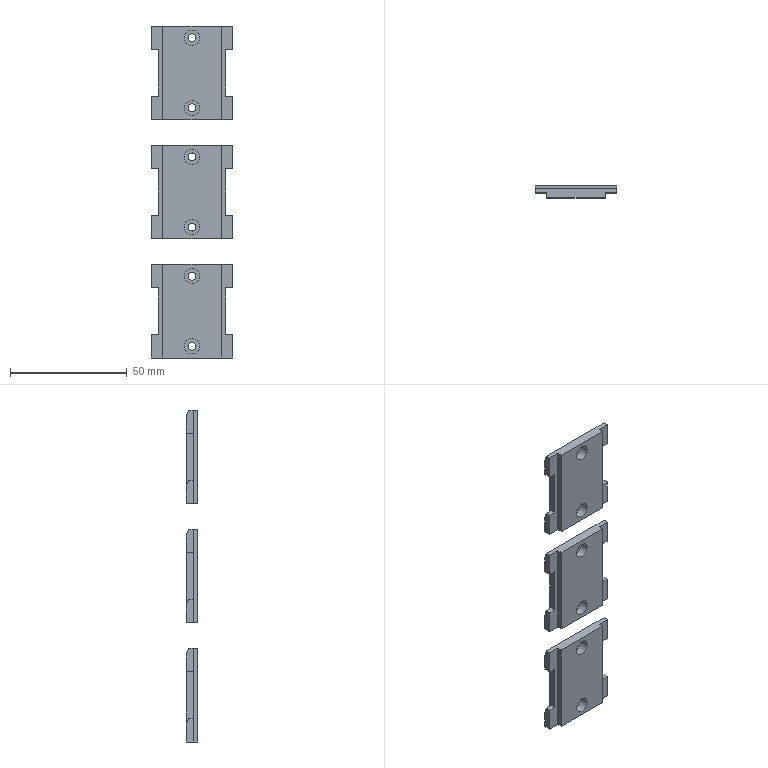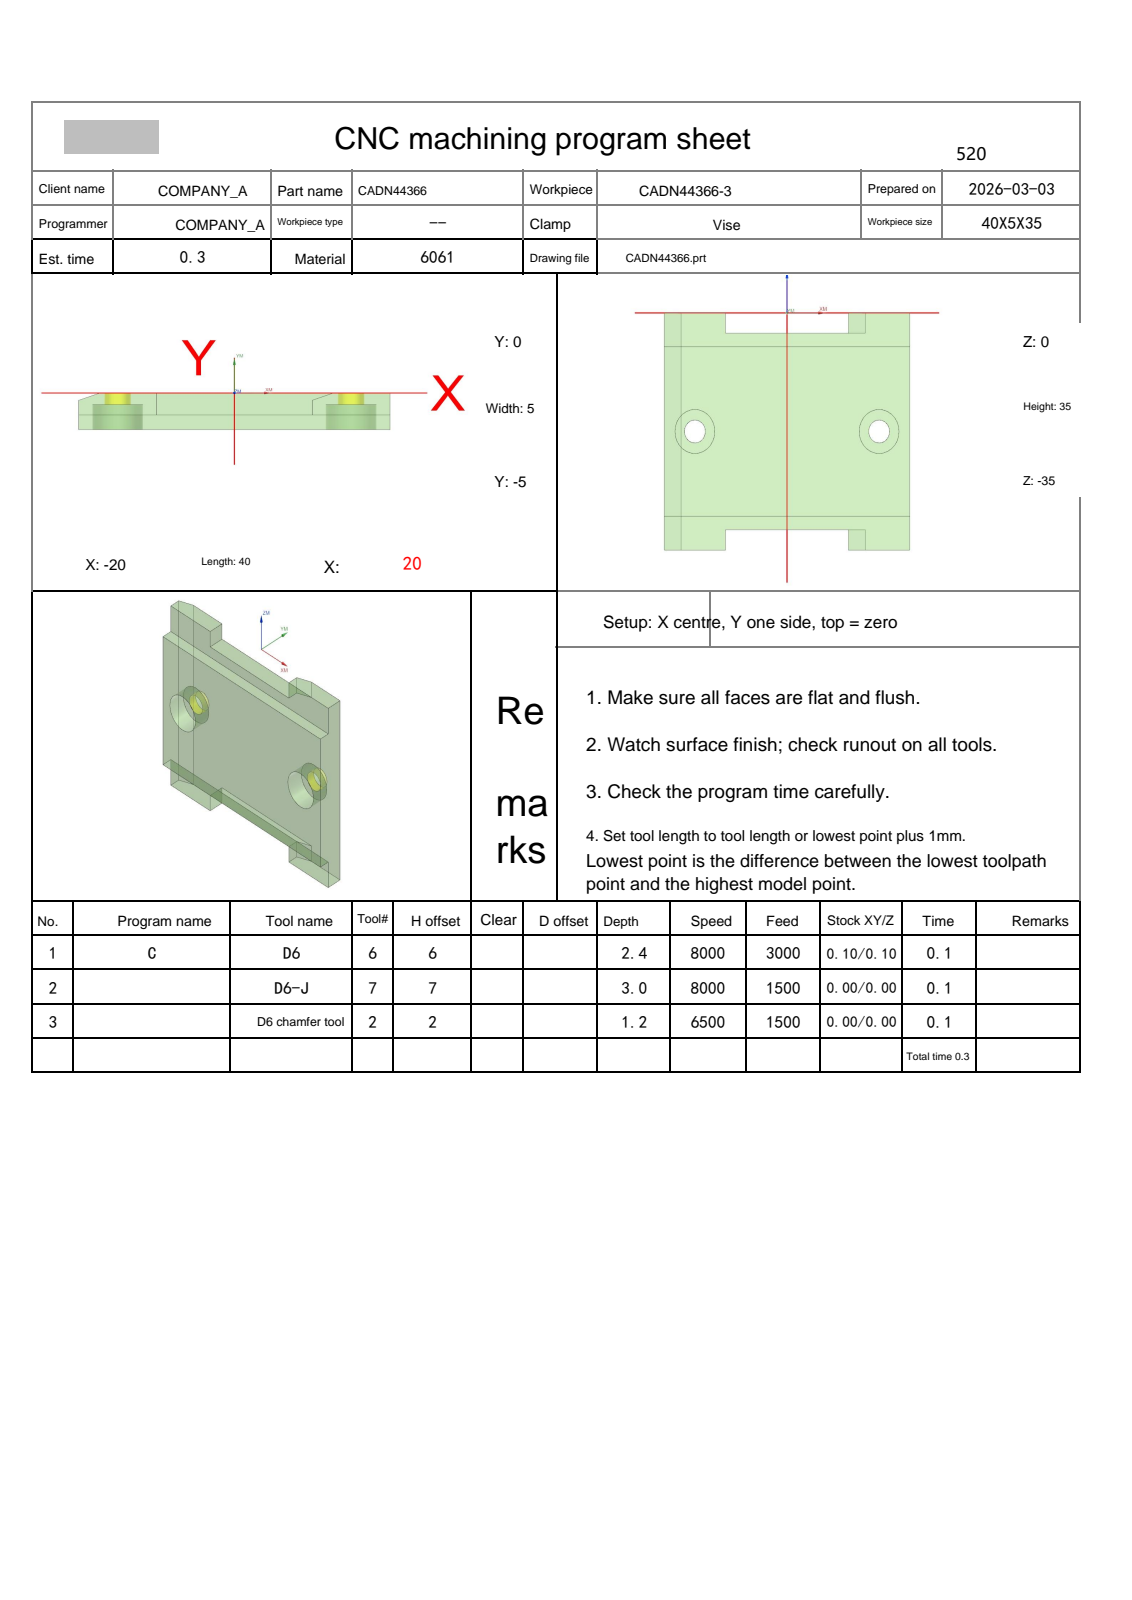NC program | NX | posted by the shop | part box 35 x 5 x 142 mm
Whole program:
%
O0001
(Machine time: 0.80 MIN)
(===Total Tool:3===)
(T6=D6      D=6.   R=0.   D-  H06 Z=-2.4  )
(T7=D6-J    D=6.   R=0.   D7  H07 Z=-3.   )
(T2=D6 chamfer tool   D=6.   R=0.   D-  H02 Z=-1.2  )
G80 G90 G17 G49 G40
G91 G28 Z0
M01
N1 T06 M06
(D6  D=6. R=0. H=06 ce=0.10 di=0.10)
G00 G90 G54 X6.9 Y-8.254 M03 S8000
G43 H06 Z50.
M08
Z-.6
G01 Y-3. F3000.
Y-1.
G02 X8.94 Y1.913 I3.1 J0.0
G01 X11.687 Y2.913
X20.406 Y6.086
G00 Z-1.2
G01 X11.687 Y2.913
X8.94 Y1.913
G03 X6.9 Y-1. I1.06 J-2.913
G01 Y-3.
Y-8.254
G00 Z-1.8
G01 Y-3.
Y-1.
G02 X8.94 Y1.913 I3.1 J0.0
G01 X11.687 Y2.913
X20.406 Y6.086
G00 Z-2.4
G01 X11.687 Y2.913
X8.94 Y1.913
G03 X6.9 Y-1. I1.06 J-2.913
G01 Y-3.
Y-8.254
G00 Z50.
X-6.9 Y5.254
Z-.6
G01 Y0.0
Y-3.
Y-8.254
G00 Z-1.2
G01 Y-3.
Y0.0
Y5.254
G00 Z-1.8
G01 Y0.0
Y-3.
Y-8.254
G00 Z-2.4
G01 Y-3.
Y0.0
Y5.254
G00 Z50.
G91 G28 Z0.0
M05
M09
G91 G28 Z0.0
M01
N2 T07 M06
(D6-J  D=6. R=0. H=07 ce=0.40 di=0.00)
G00 G90 G54 X1.2 Y-7.2 M03 S7000
G43 H07 Z10.4
M08
Z-1.5
G01 Z-3. F1500.
Y-4.8
G03 X0.0 Y-3.6 I-1.2 J0.0
G01 X-6.001
G02 X-6.6 Y-3.001 I.001 J.6
G01 Y.001
G02 X-6.001 Y.6 I.6 J-.001
G01 X6.001
G02 X6.6 Y.001 I-.001 J-.6
G01 Y-3.001
G02 X6.001 Y-3.6 I-.6 J.001
G01 X0.0
X-1.
G03 X-2.2 Y-4.8 I0.0 J-1.2
G01 Y-7.2
Z-1.5
G00 Z10.4
G00 G90 X-5.6 Y4.2 M03 S8000
Z10.011
Z-2.
G01 Z-3. F1000.
G41 D07
X-5.8
G03 X-7. Y3. I0.0 J-1.2
G01 Y-6.
G03 X-5.8 Y-7.2 I1.2 J0.0
G01 G40 X-5.6
Z-2.
G00 X5.6
G01 Z-3.
G41 D07
X5.8
G03 X7. Y-6. I0.0 J1.2
G01 Y1.101
X12.21 Y2.997
G03 X13. Y4.125 I-.41 J1.128
G01 X12.997 Y4.2
G40 X12.985 Y4.4
Z-2.
G00 Z10.011
G91 G28 Z0.0
M05
M09
G91 G28 Z0.0
M01
N3 T02 M06
(D6 chamfer tool  D=6. R=0. H=02 ce=0.00 di=0.00)
G00 G90 G54 X-14.614 Y-4.227 M03 S6500
G43 H02 Z50.
M08
Z.172
G01 Z-1.2 F1500.
G03 X-14.9 Y-4.027 I-1.286 J-1.532
G01 X-14.946 Y-3.997
X-15. Y-4.
X-20.
G02 X-21. Y-3. I0.0 J1.
G01 Y-1.
G02 X-20.342 Y-.06 I1. J0.0
G01 X-17.595 Y.94
X-17.426 Y.985
X-17.253 Y1.
X-10.
G02 X-9. Y0.0 I0.0 J-1.
G01 Y-3.
G02 X-10. Y-4. I-1. J0.0
G01 X-15.
X-15.054 Y-3.997
X-15.1 Y-4.027
G03 X-15.386 Y-4.227 I1. J-1.732
G01 Z.172
G00 Z10.
X15.386
Z.172
G01 Z-1.2
G03 X15.1 Y-4.027 I-1.286 J-1.532
G01 X15.054 Y-3.997
X15. Y-4.
X10.
G02 X9. Y-3. I0.0 J1.
G01 Y-1.
G02 X9.658 Y-.06 I1. J0.0
G01 X12.405 Y.94
X12.574 Y.985
X12.747 Y1.
X20.
G02 X21. Y0.0 I0.0 J-1.
G01 Y-3.
G02 X20. Y-4. I-1. J0.0
G01 X15.
X14.946 Y-3.997
X14.9 Y-4.027
G03 X14.614 Y-4.227 I1. J-1.732
G01 Z.172
G00 Z50.
M05
M09
G91 G28 Z0.0
G91 G28 Y0.0
M30
%